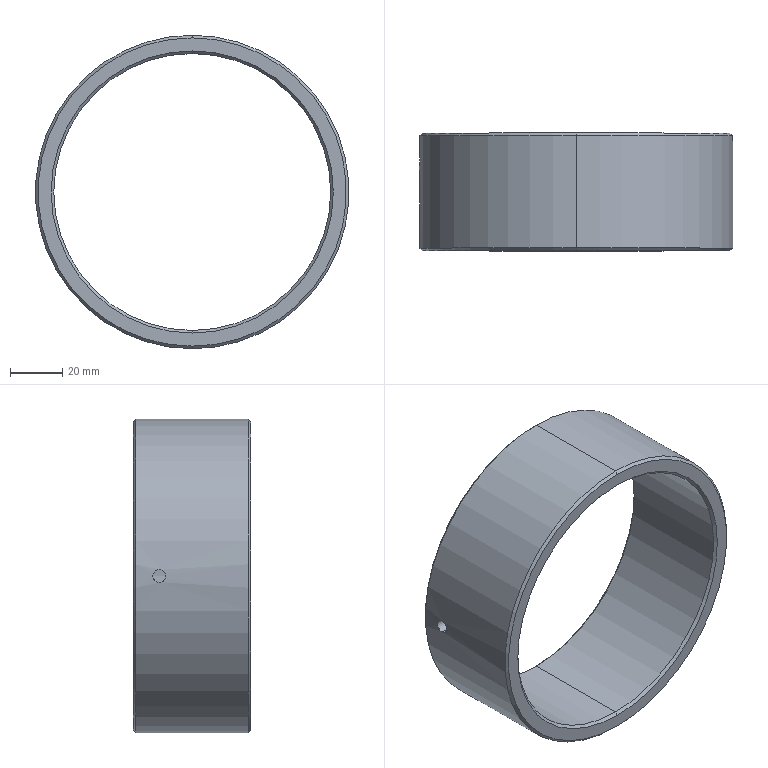Part | STEP file | PN_0001 Snap-ring locating sleeve (for centring) | 1 solid | 16 faces | box 120 x 45 x 120 mm | volume 110978 mm3 | cone 8 | cylinder 6 | plane 2 | commonest cylinder face diameters 5 x2 106 x2 120 x2